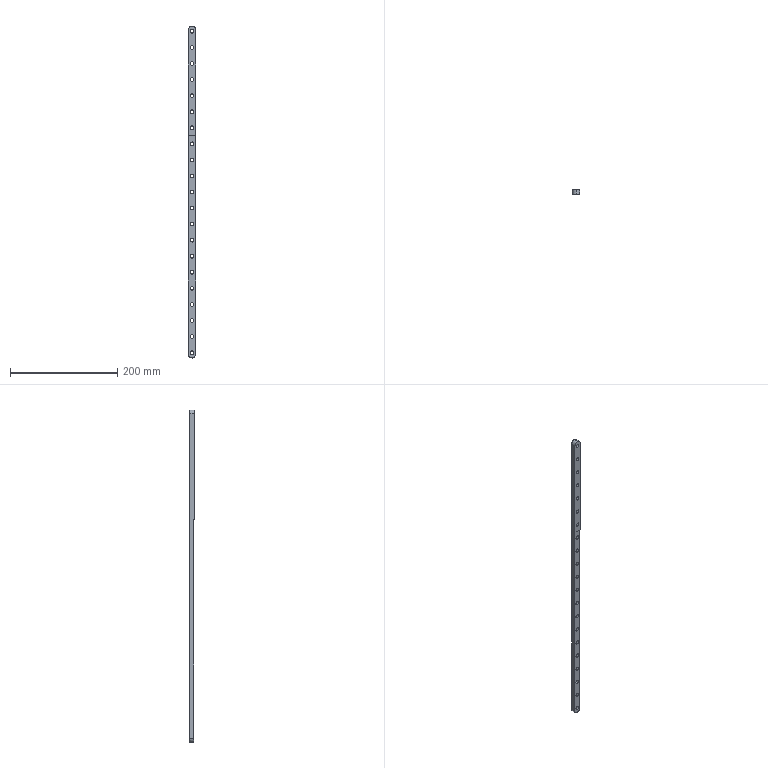Part | SolidWorks | features ICE 2, Extrusion 1, Fillet 1, HoleWzd 1, LPattern 1 | 1 solid | 117 faces | box 14 x 9 x 620 mm | volume 64305 mm3 | cylinder 46 | cone 42 | plane 29 | commonest cylinder face diameters 6.8 x42 14 x4